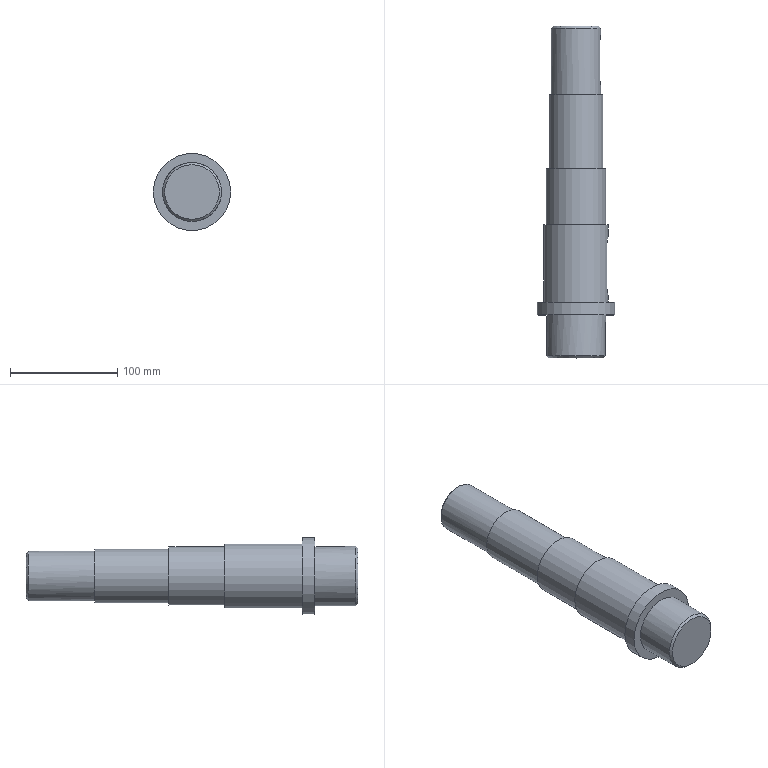Part | NX | features DATUM_CSYS 9, EXTRUDE 8, SKETCH 8, BLEND 2, CHAMFER 1 | 1 solid | 25 faces | box 72 x 309 x 72 mm | volume 701364 mm3 | plane 13 | cylinder 10 | cone 2 | commonest cylinder face diameters 12 x2 18 x2 55 x2 46.2 x1 50 x1 60 x1
STEP:
#1=CARTESIAN_POINT('',(0.,176.,25.));
#2=VERTEX_POINT('',#1);
#3=CARTESIAN_POINT('',(0.,176.,0.));
#4=DIRECTION('',(0.,1.,0.));
#5=DIRECTION('',(0.,0.,1.));
#6=AXIS2_PLACEMENT_3D('',#3,#4,#5);
#7=CIRCLE('',#6,25.);
#8=EDGE_CURVE('',#2,#2,#7,.T.);
#9=ORIENTED_EDGE('',*,*,#8,.T.);
#10=EDGE_LOOP('',(#9));
#11=FACE_BOUND('',#10,.T.);
#12=CARTESIAN_POINT('',(0.,245.,25.));
#13=VERTEX_POINT('',#12);
#14=CARTESIAN_POINT('',(0.,245.,0.));
#15=DIRECTION('',(0.,1.,0.));
#16=DIRECTION('',(0.,0.,1.));
#17=AXIS2_PLACEMENT_3D('',#14,#15,#16);
#18=CIRCLE('',#17,25.);
#19=EDGE_CURVE('',#13,#13,#18,.F.);
#20=ORIENTED_EDGE('',*,*,#19,.T.);
#21=EDGE_LOOP('',(#20));
#22=FACE_BOUND('',#21,.T.);
#23=CARTESIAN_POINT('',(0.,309.,0.));
#24=DIRECTION('',(0.,-1.,0.));
#25=DIRECTION('',(0.,0.,-1.));
#26=AXIS2_PLACEMENT_3D('',#23,#24,#25);
#27=CYLINDRICAL_SURFACE('',#26,25.);
#28=ADVANCED_FACE('',(#11,#22),#27,.T.);
#29=CARTESIAN_POINT('',(0.,2.,-27.5));
#30=VERTEX_POINT('',#29);
#31=CARTESIAN_POINT('',(0.,2.,0.));
#32=DIRECTION('',(0.,-1.,0.));
#33=DIRECTION('',(0.,0.,-1.));
#34=AXIS2_PLACEMENT_3D('',#31,#32,#33);
#35=CIRCLE('',#34,27.5);
#36=EDGE_CURVE('',#30,#30,#35,.F.);
#37=ORIENTED_EDGE('',*,*,#36,.T.);
#38=EDGE_LOOP('',(#37));
#39=FACE_BOUND('',#38,.T.);
#40=CARTESIAN_POINT('',(27.5,40.,0.));
#41=VERTEX_POINT('',#40);
#42=CARTESIAN_POINT('',(0.,40.,0.));
#43=DIRECTION('',(0.,-1.,0.));
#44=DIRECTION('',(1.,0.,0.));
#45=AXIS2_PLACEMENT_3D('',#42,#43,#44);
#46=CIRCLE('',#45,27.5);
#47=EDGE_CURVE('',#41,#41,#46,.T.);
#48=ORIENTED_EDGE('',*,*,#47,.T.);
#49=EDGE_LOOP('',(#48));
#50=FACE_BOUND('',#49,.T.);
#51=CARTESIAN_POINT('',(0.,40.,0.));
#52=DIRECTION('',(0.,-1.,0.));
#53=DIRECTION('',(0.,0.,-1.));
#54=AXIS2_PLACEMENT_3D('',#51,#52,#53);
#55=CYLINDRICAL_SURFACE('',#54,27.5);
#56=ADVANCED_FACE('',(#39,#50),#55,.T.);
#57=CARTESIAN_POINT('',(0.,0.,-25.5));
#58=VERTEX_POINT('',#57);
#59=CARTESIAN_POINT('',(0.,0.,0.));
#60=DIRECTION('',(0.,-1.,0.));
#61=DIRECTION('',(0.,0.,-1.));
#62=AXIS2_PLACEMENT_3D('',#59,#60,#61);
#63=CIRCLE('',#62,25.5);
#64=EDGE_CURVE('',#58,#58,#63,.T.);
#65=ORIENTED_EDGE('',*,*,#64,.T.);
#66=EDGE_LOOP('',(#65));
#67=FACE_BOUND('',#66,.T.);
#68=CARTESIAN_POINT('',(0.,0.,0.));
#69=DIRECTION('',(0.,-1.,0.));
#70=DIRECTION('',(0.,0.,-1.));
#71=AXIS2_PLACEMENT_3D('',#68,#69,#70);
#72=PLANE('',#71);
#73=ADVANCED_FACE('',(#67),#72,.T.);
#74=CARTESIAN_POINT('',(36.,52.,0.));
#75=VERTEX_POINT('',#74);
#76=CARTESIAN_POINT('',(0.,52.,0.));
#77=DIRECTION('',(0.,1.,0.));
#78=DIRECTION('',(1.,0.,0.));
#79=AXIS2_PLACEMENT_3D('',#76,#77,#78);
#80=CIRCLE('',#79,36.);
#81=EDGE_CURVE('',#75,#75,#80,.T.);
#82=ORIENTED_EDGE('',*,*,#81,.F.);
#83=EDGE_LOOP('',(#82));
#84=FACE_BOUND('',#83,.T.);
#85=CARTESIAN_POINT('',(36.,40.,0.));
#86=VERTEX_POINT('',#85);
#87=CARTESIAN_POINT('',(0.,40.,0.));
#88=DIRECTION('',(0.,1.,0.));
#89=DIRECTION('',(1.,0.,0.));
#90=AXIS2_PLACEMENT_3D('',#87,#88,#89);
#91=CIRCLE('',#90,36.);
#92=EDGE_CURVE('',#86,#86,#91,.T.);
#93=ORIENTED_EDGE('',*,*,#92,.T.);
#94=EDGE_LOOP('',(#93));
#95=FACE_BOUND('',#94,.T.);
#96=CARTESIAN_POINT('',(0.,52.,0.));
#97=DIRECTION('',(0.,-1.,0.));
#98=DIRECTION('',(0.,0.,-1.));
#99=AXIS2_PLACEMENT_3D('',#96,#97,#98);
#100=CYLINDRICAL_SURFACE('',#99,36.);
#101=ADVANCED_FACE('',(#84,#95),#100,.T.);
#102=CARTESIAN_POINT('',(30.,52.,0.));
#103=VERTEX_POINT('',#102);
#104=CARTESIAN_POINT('',(0.,52.,0.));
#105=DIRECTION('',(0.,1.,0.));
#106=DIRECTION('',(1.,0.,0.));
#107=AXIS2_PLACEMENT_3D('',#104,#105,#106);
#108=CIRCLE('',#107,30.);
#109=EDGE_CURVE('',#103,#103,#108,.T.);
#110=ORIENTED_EDGE('',*,*,#109,.F.);
#111=EDGE_LOOP('',(#110));
#112=FACE_BOUND('',#111,.T.);
#113=ORIENTED_EDGE('',*,*,#81,.T.);
#114=EDGE_LOOP('',(#113));
#115=FACE_BOUND('',#114,.T.);
#116=CARTESIAN_POINT('',(0.,52.,0.));
#117=DIRECTION('',(0.,1.,0.));
#118=DIRECTION('',(0.,0.,1.));
#119=AXIS2_PLACEMENT_3D('',#116,#117,#118);
#120=PLANE('',#119);
#121=ADVANCED_FACE('',(#112,#115),#120,.T.);
#122=ORIENTED_EDGE('',*,*,#47,.F.);
#123=EDGE_LOOP('',(#122));
#124=FACE_BOUND('',#123,.T.);
#125=ORIENTED_EDGE('',*,*,#92,.F.);
#126=EDGE_LOOP('',(#125));
#127=FACE_BOUND('',#126,.T.);
#128=CARTESIAN_POINT('',(0.,40.,0.));
#129=DIRECTION('',(0.,1.,0.));
#130=DIRECTION('',(0.,0.,1.));
#131=AXIS2_PLACEMENT_3D('',#128,#129,#130);
#132=PLANE('',#131);
#133=ADVANCED_FACE('',(#124,#127),#132,.F.);
#134=CARTESIAN_POINT('',(28.618,67.,-9.));
#135=VERTEX_POINT('',#134);
#136=CARTESIAN_POINT('',(28.618,104.,-9.));
#137=VERTEX_POINT('',#136);
#138=CARTESIAN_POINT('',(28.618,124.,-9.));
#139=DIRECTION('',(0.,-1.,0.));
#140=VECTOR('',#139,1000.);
#141=LINE('',#138,#140);
#142=EDGE_CURVE('',#135,#137,#141,.F.);
#143=ORIENTED_EDGE('',*,*,#142,.F.);
#144=CARTESIAN_POINT('',(28.618,67.,9.));
#145=VERTEX_POINT('',#144);
#146=CARTESIAN_POINT('',(28.618,67.,-9.));
#147=CARTESIAN_POINT('',(28.618,64.608,-9.));
#148=CARTESIAN_POINT('',(29.137,61.137,-7.52));
#149=CARTESIAN_POINT('',(29.85,58.482,-3.564));
#150=CARTESIAN_POINT('',(30.158,57.514,1.198));
#151=CARTESIAN_POINT('',(29.33,59.964,7.043));
#152=CARTESIAN_POINT('',(28.618,64.608,9.));
#153=CARTESIAN_POINT('',(28.618,67.,9.));
#154=B_SPLINE_CURVE_WITH_KNOTS('',3,(#146,#147,#148,#149,#150,#151,#152,#153),.UNSPECIFIED.,.F.,.F.,(4,1,1,1,1,4),(-0.01414,-0.007071,-0.003535,0.000000131,0.007071,0.01414),.UNSPECIFIED.);
#155=EDGE_CURVE('',#135,#145,#154,.T.);
#156=ORIENTED_EDGE('',*,*,#155,.T.);
#157=CARTESIAN_POINT('',(28.618,104.,9.));
#158=VERTEX_POINT('',#157);
#159=CARTESIAN_POINT('',(28.618,124.,9.));
#160=DIRECTION('',(0.,-1.,0.));
#161=VECTOR('',#160,1000.);
#162=LINE('',#159,#161);
#163=EDGE_CURVE('',#145,#158,#162,.F.);
#164=ORIENTED_EDGE('',*,*,#163,.T.);
#165=CARTESIAN_POINT('',(28.618,104.,9.));
#166=CARTESIAN_POINT('',(28.618,106.392,9.));
#167=CARTESIAN_POINT('',(29.137,109.863,7.52));
#168=CARTESIAN_POINT('',(29.85,112.518,3.564));
#169=CARTESIAN_POINT('',(30.158,113.486,-1.198));
#170=CARTESIAN_POINT('',(29.33,111.036,-7.043));
#171=CARTESIAN_POINT('',(28.618,106.392,-9.));
#172=CARTESIAN_POINT('',(28.618,104.,-9.));
#173=B_SPLINE_CURVE_WITH_KNOTS('',3,(#165,#166,#167,#168,#169,#170,#171,#172),.UNSPECIFIED.,.F.,.F.,(4,1,1,1,1,4),(-0.01414,-0.007071,-0.003535,0.000000131,0.007071,0.01414),.UNSPECIFIED.);
#174=EDGE_CURVE('',#158,#137,#173,.T.);
#175=ORIENTED_EDGE('',*,*,#174,.T.);
#176=EDGE_LOOP('',(#143,#156,#164,#175));
#177=FACE_BOUND('',#176,.T.);
#178=CARTESIAN_POINT('',(30.,124.,0.));
#179=VERTEX_POINT('',#178);
#180=CARTESIAN_POINT('',(0.,124.,0.));
#181=DIRECTION('',(0.,1.,0.));
#182=DIRECTION('',(1.,0.,0.));
#183=AXIS2_PLACEMENT_3D('',#180,#181,#182);
#184=CIRCLE('',#183,30.);
#185=EDGE_CURVE('',#179,#179,#184,.T.);
#186=ORIENTED_EDGE('',*,*,#185,.F.);
#187=EDGE_LOOP('',(#186));
#188=FACE_BOUND('',#187,.T.);
#189=ORIENTED_EDGE('',*,*,#109,.T.);
#190=EDGE_LOOP('',(#189));
#191=FACE_BOUND('',#190,.T.);
#192=CARTESIAN_POINT('',(0.,124.,0.));
#193=DIRECTION('',(0.,-1.,0.));
#194=DIRECTION('',(0.,0.,-1.));
#195=AXIS2_PLACEMENT_3D('',#192,#193,#194);
#196=CYLINDRICAL_SURFACE('',#195,30.);
#197=ADVANCED_FACE('',(#177,#188,#191),#196,.T.);
#198=CARTESIAN_POINT('',(27.5,124.,0.));
#199=VERTEX_POINT('',#198);
#200=CARTESIAN_POINT('',(0.,124.,0.));
#201=DIRECTION('',(0.,1.,0.));
#202=DIRECTION('',(1.,0.,0.));
#203=AXIS2_PLACEMENT_3D('',#200,#201,#202);
#204=CIRCLE('',#203,27.5);
#205=EDGE_CURVE('',#199,#199,#204,.T.);
#206=ORIENTED_EDGE('',*,*,#205,.F.);
#207=EDGE_LOOP('',(#206));
#208=FACE_BOUND('',#207,.T.);
#209=ORIENTED_EDGE('',*,*,#185,.T.);
#210=EDGE_LOOP('',(#209));
#211=FACE_BOUND('',#210,.T.);
#212=CARTESIAN_POINT('',(0.,124.,0.));
#213=DIRECTION('',(0.,1.,0.));
#214=DIRECTION('',(0.,0.,1.));
#215=AXIS2_PLACEMENT_3D('',#212,#213,#214);
#216=PLANE('',#215);
#217=ADVANCED_FACE('',(#208,#211),#216,.T.);
#218=CARTESIAN_POINT('',(27.5,176.,0.));
#219=VERTEX_POINT('',#218);
#220=CARTESIAN_POINT('',(0.,176.,0.));
#221=DIRECTION('',(0.,1.,0.));
#222=DIRECTION('',(1.,0.,0.));
#223=AXIS2_PLACEMENT_3D('',#220,#221,#222);
#224=CIRCLE('',#223,27.5);
#225=EDGE_CURVE('',#219,#219,#224,.T.);
#226=ORIENTED_EDGE('',*,*,#225,.F.);
#227=EDGE_LOOP('',(#226));
#228=FACE_BOUND('',#227,.T.);
#229=ORIENTED_EDGE('',*,*,#205,.T.);
#230=EDGE_LOOP('',(#229));
#231=FACE_BOUND('',#230,.T.);
#232=CARTESIAN_POINT('',(0.,176.,0.));
#233=DIRECTION('',(0.,-1.,0.));
#234=DIRECTION('',(0.,0.,-1.));
#235=AXIS2_PLACEMENT_3D('',#232,#233,#234);
#236=CYLINDRICAL_SURFACE('',#235,27.5);
#237=ADVANCED_FACE('',(#228,#231),#236,.T.);
#238=ORIENTED_EDGE('',*,*,#8,.F.);
#239=EDGE_LOOP('',(#238));
#240=FACE_BOUND('',#239,.T.);
#241=ORIENTED_EDGE('',*,*,#225,.T.);
#242=EDGE_LOOP('',(#241));
#243=FACE_BOUND('',#242,.T.);
#244=CARTESIAN_POINT('',(0.,176.,0.));
#245=DIRECTION('',(0.,1.,0.));
#246=DIRECTION('',(0.,0.,1.));
#247=AXIS2_PLACEMENT_3D('',#244,#245,#246);
#248=PLANE('',#247);
#249=ADVANCED_FACE('',(#240,#243),#248,.T.);
#250=CARTESIAN_POINT('',(0.,307.,-23.1));
#251=VERTEX_POINT('',#250);
#252=CARTESIAN_POINT('',(0.,307.,0.));
#253=DIRECTION('',(0.,-1.,0.));
#254=DIRECTION('',(0.,0.,-1.));
#255=AXIS2_PLACEMENT_3D('',#252,#253,#254);
#256=CIRCLE('',#255,23.1);
#257=EDGE_CURVE('',#251,#251,#256,.T.);
#258=ORIENTED_EDGE('',*,*,#257,.T.);
#259=EDGE_LOOP('',(#258));
#260=FACE_BOUND('',#259,.T.);
#261=CARTESIAN_POINT('',(22.307,295.,6.));
#262=VERTEX_POINT('',#261);
#263=CARTESIAN_POINT('',(22.307,259.,6.));
#264=VERTEX_POINT('',#263);
#265=CARTESIAN_POINT('',(22.307,245.,6.));
#266=DIRECTION('',(0.,1.,0.));
#267=VECTOR('',#266,1000.);
#268=LINE('',#265,#267);
#269=EDGE_CURVE('',#262,#264,#268,.F.);
#270=ORIENTED_EDGE('',*,*,#269,.F.);
#271=CARTESIAN_POINT('',(22.307,295.,-6.));
#272=VERTEX_POINT('',#271);
#273=CARTESIAN_POINT('',(22.307,295.,6.));
#274=CARTESIAN_POINT('',(22.307,296.592,6.));
#275=CARTESIAN_POINT('',(22.71,299.687,4.704));
#276=CARTESIAN_POINT('',(23.295,301.656,-0.00125));
#277=CARTESIAN_POINT('',(22.711,299.691,-4.7));
#278=CARTESIAN_POINT('',(22.307,296.592,-6.));
#279=CARTESIAN_POINT('',(22.307,295.,-6.));
#280=B_SPLINE_CURVE_WITH_KNOTS('',3,(#273,#274,#275,#276,#277,#278,#279),.UNSPECIFIED.,.F.,.F.,(4,1,1,1,4),(-0.009413,-0.004707,0.000000114,0.004707,0.009414),.UNSPECIFIED.);
#281=EDGE_CURVE('',#262,#272,#280,.T.);
#282=ORIENTED_EDGE('',*,*,#281,.T.);
#283=CARTESIAN_POINT('',(22.307,259.,-6.));
#284=VERTEX_POINT('',#283);
#285=CARTESIAN_POINT('',(22.307,245.,-6.));
#286=DIRECTION('',(0.,1.,0.));
#287=VECTOR('',#286,1000.);
#288=LINE('',#285,#287);
#289=EDGE_CURVE('',#272,#284,#288,.F.);
#290=ORIENTED_EDGE('',*,*,#289,.T.);
#291=CARTESIAN_POINT('',(22.307,259.,-6.));
#292=CARTESIAN_POINT('',(22.307,257.408,-6.));
#293=CARTESIAN_POINT('',(22.71,254.313,-4.704));
#294=CARTESIAN_POINT('',(23.295,252.344,0.00125));
#295=CARTESIAN_POINT('',(22.711,254.309,4.7));
#296=CARTESIAN_POINT('',(22.307,257.408,6.));
#297=CARTESIAN_POINT('',(22.307,259.,6.));
#298=B_SPLINE_CURVE_WITH_KNOTS('',3,(#291,#292,#293,#294,#295,#296,#297),.UNSPECIFIED.,.F.,.F.,(4,1,1,1,4),(-0.009413,-0.004707,0.000000114,0.004707,0.009414),.UNSPECIFIED.);
#299=EDGE_CURVE('',#284,#264,#298,.T.);
#300=ORIENTED_EDGE('',*,*,#299,.T.);
#301=EDGE_LOOP('',(#270,#282,#290,#300));
#302=FACE_BOUND('',#301,.T.);
#303=CARTESIAN_POINT('',(23.1,245.,0.));
#304=VERTEX_POINT('',#303);
#305=CARTESIAN_POINT('',(0.,245.,0.));
#306=DIRECTION('',(0.,1.,0.));
#307=DIRECTION('',(1.,0.,0.));
#308=AXIS2_PLACEMENT_3D('',#305,#306,#307);
#309=CIRCLE('',#308,23.1);
#310=EDGE_CURVE('',#304,#304,#309,.F.);
#311=ORIENTED_EDGE('',*,*,#310,.F.);
#312=EDGE_LOOP('',(#311));
#313=FACE_BOUND('',#312,.T.);
#314=CARTESIAN_POINT('',(0.,245.,0.));
#315=DIRECTION('',(0.,1.,0.));
#316=DIRECTION('',(0.,0.,1.));
#317=AXIS2_PLACEMENT_3D('',#314,#315,#316);
#318=CYLINDRICAL_SURFACE('',#317,23.1);
#319=ADVANCED_FACE('',(#260,#302,#313),#318,.T.);
#320=ORIENTED_EDGE('',*,*,#19,.F.);
#321=EDGE_LOOP('',(#320));
#322=FACE_BOUND('',#321,.T.);
#323=ORIENTED_EDGE('',*,*,#310,.T.);
#324=EDGE_LOOP('',(#323));
#325=FACE_BOUND('',#324,.T.);
#326=CARTESIAN_POINT('',(0.,245.,0.));
#327=DIRECTION('',(0.,1.,0.));
#328=DIRECTION('',(0.,0.,1.));
#329=AXIS2_PLACEMENT_3D('',#326,#327,#328);
#330=PLANE('',#329);
#331=ADVANCED_FACE('',(#322,#325),#330,.T.);
#332=CARTESIAN_POINT('',(0.,309.,-21.1));
#333=VERTEX_POINT('',#332);
#334=CARTESIAN_POINT('',(0.,309.,0.));
#335=DIRECTION('',(0.,-1.,0.));
#336=DIRECTION('',(0.,0.,-1.));
#337=AXIS2_PLACEMENT_3D('',#334,#335,#336);
#338=CIRCLE('',#337,21.1);
#339=EDGE_CURVE('',#333,#333,#338,.F.);
#340=ORIENTED_EDGE('',*,*,#339,.T.);
#341=EDGE_LOOP('',(#340));
#342=FACE_BOUND('',#341,.T.);
#343=CARTESIAN_POINT('',(0.,309.,0.));
#344=DIRECTION('',(0.,-1.,0.));
#345=DIRECTION('',(0.,0.,-1.));
#346=AXIS2_PLACEMENT_3D('',#343,#344,#345);
#347=PLANE('',#346);
#348=ADVANCED_FACE('',(#342),#347,.F.);
#349=CARTESIAN_POINT('',(22.,67.,9.));
#350=VERTEX_POINT('',#349);
#351=CARTESIAN_POINT('',(22.,104.,9.));
#352=VERTEX_POINT('',#351);
#353=CARTESIAN_POINT('',(22.,113.,9.));
#354=DIRECTION('',(0.,-1.,0.));
#355=VECTOR('',#354,1000.);
#356=LINE('',#353,#355);
#357=EDGE_CURVE('',#350,#352,#356,.F.);
#358=ORIENTED_EDGE('',*,*,#357,.T.);
#359=CARTESIAN_POINT('',(0.,104.,9.));
#360=DIRECTION('',(1.,0.,0.));
#361=VECTOR('',#360,1000.);
#362=LINE('',#359,#361);
#363=EDGE_CURVE('',#352,#158,#362,.T.);
#364=ORIENTED_EDGE('',*,*,#363,.T.);
#365=ORIENTED_EDGE('',*,*,#163,.F.);
#366=CARTESIAN_POINT('',(0.,67.,9.));
#367=DIRECTION('',(-1.,0.,0.));
#368=VECTOR('',#367,1000.);
#369=LINE('',#366,#368);
#370=EDGE_CURVE('',#145,#350,#369,.T.);
#371=ORIENTED_EDGE('',*,*,#370,.T.);
#372=EDGE_LOOP('',(#358,#364,#365,#371));
#373=FACE_BOUND('',#372,.T.);
#374=CARTESIAN_POINT('',(0.,0.,9.));
#375=DIRECTION('',(0.,0.,1.));
#376=DIRECTION('',(1.,0.,0.));
#377=AXIS2_PLACEMENT_3D('',#374,#375,#376);
#378=PLANE('',#377);
#379=ADVANCED_FACE('',(#373),#378,.F.);
#380=ORIENTED_EDGE('',*,*,#142,.T.);
#381=CARTESIAN_POINT('',(22.,104.,-9.));
#382=VERTEX_POINT('',#381);
#383=CARTESIAN_POINT('',(22.,104.,-9.));
#384=DIRECTION('',(1.,0.,0.));
#385=VECTOR('',#384,1000.);
#386=LINE('',#383,#385);
#387=EDGE_CURVE('',#137,#382,#386,.F.);
#388=ORIENTED_EDGE('',*,*,#387,.T.);
#389=CARTESIAN_POINT('',(22.,67.,-9.));
#390=VERTEX_POINT('',#389);
#391=CARTESIAN_POINT('',(22.,113.,-9.));
#392=DIRECTION('',(0.,-1.,0.));
#393=VECTOR('',#392,1000.);
#394=LINE('',#391,#393);
#395=EDGE_CURVE('',#390,#382,#394,.F.);
#396=ORIENTED_EDGE('',*,*,#395,.F.);
#397=CARTESIAN_POINT('',(28.618,67.,-9.));
#398=DIRECTION('',(-1.,0.,0.));
#399=VECTOR('',#398,1000.);
#400=LINE('',#397,#399);
#401=EDGE_CURVE('',#390,#135,#400,.F.);
#402=ORIENTED_EDGE('',*,*,#401,.T.);
#403=EDGE_LOOP('',(#380,#388,#396,#402));
#404=FACE_BOUND('',#403,.T.);
#405=CARTESIAN_POINT('',(0.,0.,-9.));
#406=DIRECTION('',(0.,0.,1.));
#407=DIRECTION('',(1.,0.,0.));
#408=AXIS2_PLACEMENT_3D('',#405,#406,#407);
#409=PLANE('',#408);
#410=ADVANCED_FACE('',(#404),#409,.T.);
#411=ORIENTED_EDGE('',*,*,#395,.T.);
#412=CARTESIAN_POINT('',(22.,104.,0.));
#413=DIRECTION('',(1.,0.,0.));
#414=DIRECTION('',(0.,0.,-1.));
#415=AXIS2_PLACEMENT_3D('',#412,#413,#414);
#416=CIRCLE('',#415,9.);
#417=EDGE_CURVE('',#382,#352,#416,.T.);
#418=ORIENTED_EDGE('',*,*,#417,.T.);
#419=ORIENTED_EDGE('',*,*,#357,.F.);
#420=CARTESIAN_POINT('',(22.,67.,0.));
#421=DIRECTION('',(1.,0.,0.));
#422=DIRECTION('',(0.,0.,-1.));
#423=AXIS2_PLACEMENT_3D('',#420,#421,#422);
#424=CIRCLE('',#423,9.);
#425=EDGE_CURVE('',#350,#390,#424,.T.);
#426=ORIENTED_EDGE('',*,*,#425,.T.);
#427=EDGE_LOOP('',(#411,#418,#419,#426));
#428=FACE_BOUND('',#427,.T.);
#429=CARTESIAN_POINT('',(22.,113.,9.));
#430=DIRECTION('',(1.,0.,0.));
#431=DIRECTION('',(0.,0.,-1.));
#432=AXIS2_PLACEMENT_3D('',#429,#430,#431);
#433=PLANE('',#432);
#434=ADVANCED_FACE('',(#428),#433,.T.);
#435=ORIENTED_EDGE('',*,*,#363,.F.);
#436=ORIENTED_EDGE('',*,*,#417,.F.);
#437=ORIENTED_EDGE('',*,*,#387,.F.);
#438=ORIENTED_EDGE('',*,*,#174,.F.);
#439=EDGE_LOOP('',(#435,#436,#437,#438));
#440=FACE_BOUND('',#439,.T.);
#441=CARTESIAN_POINT('',(0.,104.,0.));
#442=DIRECTION('',(1.,0.,0.));
#443=DIRECTION('',(0.,0.,-1.));
#444=AXIS2_PLACEMENT_3D('',#441,#442,#443);
#445=CYLINDRICAL_SURFACE('',#444,9.);
#446=ADVANCED_FACE('',(#440),#445,.F.);
#447=ORIENTED_EDGE('',*,*,#425,.F.);
#448=ORIENTED_EDGE('',*,*,#370,.F.);
#449=ORIENTED_EDGE('',*,*,#155,.F.);
#450=ORIENTED_EDGE('',*,*,#401,.F.);
#451=EDGE_LOOP('',(#447,#448,#449,#450));
#452=FACE_BOUND('',#451,.T.);
#453=CARTESIAN_POINT('',(22.,67.,0.));
#454=DIRECTION('',(1.,0.,0.));
#455=DIRECTION('',(0.,0.,-1.));
#456=AXIS2_PLACEMENT_3D('',#453,#454,#455);
#457=CYLINDRICAL_SURFACE('',#456,9.);
#458=ADVANCED_FACE('',(#452),#457,.F.);
#459=CARTESIAN_POINT('',(14.,259.,-6.));
#460=VERTEX_POINT('',#459);
#461=CARTESIAN_POINT('',(14.,295.,-6.));
#462=VERTEX_POINT('',#461);
#463=CARTESIAN_POINT('',(14.,301.,-6.));
#464=DIRECTION('',(0.,-1.,0.));
#465=VECTOR('',#464,1000.);
#466=LINE('',#463,#465);
#467=EDGE_CURVE('',#460,#462,#466,.F.);
#468=ORIENTED_EDGE('',*,*,#467,.T.);
#469=CARTESIAN_POINT('',(14.,295.,6.));
#470=VERTEX_POINT('',#469);
#471=CARTESIAN_POINT('',(14.,295.,0.));
#472=DIRECTION('',(1.,0.,0.));
#473=DIRECTION('',(0.,1.,0.));
#474=AXIS2_PLACEMENT_3D('',#471,#472,#473);
#475=CIRCLE('',#474,6.);
#476=EDGE_CURVE('',#462,#470,#475,.T.);
#477=ORIENTED_EDGE('',*,*,#476,.T.);
#478=CARTESIAN_POINT('',(14.,259.,6.));
#479=VERTEX_POINT('',#478);
#480=CARTESIAN_POINT('',(14.,301.,6.));
#481=DIRECTION('',(0.,-1.,0.));
#482=VECTOR('',#481,1000.);
#483=LINE('',#480,#482);
#484=EDGE_CURVE('',#479,#470,#483,.F.);
#485=ORIENTED_EDGE('',*,*,#484,.F.);
#486=CARTESIAN_POINT('',(14.,259.,0.));
#487=DIRECTION('',(1.,0.,0.));
#488=DIRECTION('',(0.,1.,0.));
#489=AXIS2_PLACEMENT_3D('',#486,#487,#488);
#490=CIRCLE('',#489,6.);
#491=EDGE_CURVE('',#479,#460,#490,.T.);
#492=ORIENTED_EDGE('',*,*,#491,.T.);
#493=EDGE_LOOP('',(#468,#477,#485,#492));
#494=FACE_BOUND('',#493,.T.);
#495=CARTESIAN_POINT('',(14.,301.,6.));
#496=DIRECTION('',(1.,0.,0.));
#497=DIRECTION('',(0.,1.,0.));
#498=AXIS2_PLACEMENT_3D('',#495,#496,#497);
#499=PLANE('',#498);
#500=ADVANCED_FACE('',(#494),#499,.T.);
#501=ORIENTED_EDGE('',*,*,#484,.T.);
#502=CARTESIAN_POINT('',(0.,295.,6.));
#503=DIRECTION('',(1.,0.,0.));
#504=VECTOR('',#503,1000.);
#505=LINE('',#502,#504);
#506=EDGE_CURVE('',#470,#262,#505,.T.);
#507=ORIENTED_EDGE('',*,*,#506,.T.);
#508=ORIENTED_EDGE('',*,*,#269,.T.);
#509=CARTESIAN_POINT('',(0.,259.,6.));
#510=DIRECTION('',(-1.,0.,0.));
#511=VECTOR('',#510,1000.);
#512=LINE('',#509,#511);
#513=EDGE_CURVE('',#264,#479,#512,.T.);
#514=ORIENTED_EDGE('',*,*,#513,.T.);
#515=EDGE_LOOP('',(#501,#507,#508,#514));
#516=FACE_BOUND('',#515,.T.);
#517=CARTESIAN_POINT('',(0.,0.,6.));
#518=DIRECTION('',(0.,0.,1.));
#519=DIRECTION('',(1.,0.,0.));
#520=AXIS2_PLACEMENT_3D('',#517,#518,#519);
#521=PLANE('',#520);
#522=ADVANCED_FACE('',(#516),#521,.F.);
#523=ORIENTED_EDGE('',*,*,#289,.F.);
#524=CARTESIAN_POINT('',(14.,295.,-6.));
#525=DIRECTION('',(1.,0.,0.));
#526=VECTOR('',#525,1000.);
#527=LINE('',#524,#526);
#528=EDGE_CURVE('',#272,#462,#527,.F.);
#529=ORIENTED_EDGE('',*,*,#528,.T.);
#530=ORIENTED_EDGE('',*,*,#467,.F.);
#531=CARTESIAN_POINT('',(22.307,259.,-6.));
#532=DIRECTION('',(-1.,0.,0.));
#533=VECTOR('',#532,1000.);
#534=LINE('',#531,#533);
#535=EDGE_CURVE('',#460,#284,#534,.F.);
#536=ORIENTED_EDGE('',*,*,#535,.T.);
#537=EDGE_LOOP('',(#523,#529,#530,#536));
#538=FACE_BOUND('',#537,.T.);
#539=CARTESIAN_POINT('',(0.,0.,-6.));
#540=DIRECTION('',(0.,0.,1.));
#541=DIRECTION('',(1.,0.,0.));
#542=AXIS2_PLACEMENT_3D('',#539,#540,#541);
#543=PLANE('',#542);
#544=ADVANCED_FACE('',(#538),#543,.T.);
#545=ORIENTED_EDGE('',*,*,#506,.F.);
#546=ORIENTED_EDGE('',*,*,#476,.F.);
#547=ORIENTED_EDGE('',*,*,#528,.F.);
#548=ORIENTED_EDGE('',*,*,#281,.F.);
#549=EDGE_LOOP('',(#545,#546,#547,#548));
#550=FACE_BOUND('',#549,.T.);
#551=CARTESIAN_POINT('',(0.,295.,0.));
#552=DIRECTION('',(1.,0.,0.));
#553=DIRECTION('',(0.,0.,-1.));
#554=AXIS2_PLACEMENT_3D('',#551,#552,#553);
#555=CYLINDRICAL_SURFACE('',#554,6.);
#556=ADVANCED_FACE('',(#550),#555,.F.);
#557=ORIENTED_EDGE('',*,*,#491,.F.);
#558=ORIENTED_EDGE('',*,*,#513,.F.);
#559=ORIENTED_EDGE('',*,*,#299,.F.);
#560=ORIENTED_EDGE('',*,*,#535,.F.);
#561=EDGE_LOOP('',(#557,#558,#559,#560));
#562=FACE_BOUND('',#561,.T.);
#563=CARTESIAN_POINT('',(14.,259.,0.));
#564=DIRECTION('',(1.,0.,0.));
#565=DIRECTION('',(0.,0.,-1.));
#566=AXIS2_PLACEMENT_3D('',#563,#564,#565);
#567=CYLINDRICAL_SURFACE('',#566,6.);
#568=ADVANCED_FACE('',(#562),#567,.F.);
#569=ORIENTED_EDGE('',*,*,#257,.F.);
#570=EDGE_LOOP('',(#569));
#571=FACE_BOUND('',#570,.T.);
#572=ORIENTED_EDGE('',*,*,#339,.F.);
#573=EDGE_LOOP('',(#572));
#574=FACE_BOUND('',#573,.T.);
#575=CARTESIAN_POINT('',(0.,309.,0.));
#576=DIRECTION('',(0.,-1.,0.));
#577=DIRECTION('',(0.,0.,-1.));
#578=AXIS2_PLACEMENT_3D('',#575,#576,#577);
#579=CONICAL_SURFACE('',#578,21.1,0.7854);
#580=ADVANCED_FACE('',(#571,#574),#579,.T.);
#581=ORIENTED_EDGE('',*,*,#36,.F.);
#582=EDGE_LOOP('',(#581));
#583=FACE_BOUND('',#582,.T.);
#584=ORIENTED_EDGE('',*,*,#64,.F.);
#585=EDGE_LOOP('',(#584));
#586=FACE_BOUND('',#585,.T.);
#587=CARTESIAN_POINT('',(0.,0.,0.));
#588=DIRECTION('',(0.,1.,0.));
#589=DIRECTION('',(0.,0.,1.));
#590=AXIS2_PLACEMENT_3D('',#587,#588,#589);
#591=CONICAL_SURFACE('',#590,25.5,0.7854);
#592=ADVANCED_FACE('',(#583,#586),#591,.T.);
#593=CLOSED_SHELL('',(#28,#56,#73,#101,#121,#133,#197,#217,#237,#249,#319,#331,#348,#379,#410,#434,#446,#458,#500,#522,#544,#556,#568,#580,#592));
#594=MANIFOLD_SOLID_BREP('',#593);
#595=(LENGTH_UNIT()NAMED_UNIT(*)SI_UNIT(.MILLI.,.METRE.));
#596=UNCERTAINTY_MEASURE_WITH_UNIT(LENGTH_MEASURE(0.0508),#595,'','');
#597=(NAMED_UNIT(*)PLANE_ANGLE_UNIT()SI_UNIT($,.RADIAN.));
#598=(NAMED_UNIT(*)SI_UNIT($,.STERADIAN.)SOLID_ANGLE_UNIT());
#599=(GEOMETRIC_REPRESENTATION_CONTEXT(3)GLOBAL_UNCERTAINTY_ASSIGNED_CONTEXT((#596))GLOBAL_UNIT_ASSIGNED_CONTEXT((#595,#597,#598))REPRESENTATION_CONTEXT('',''));
#600=ADVANCED_BREP_SHAPE_REPRESENTATION('',(#594),#599);